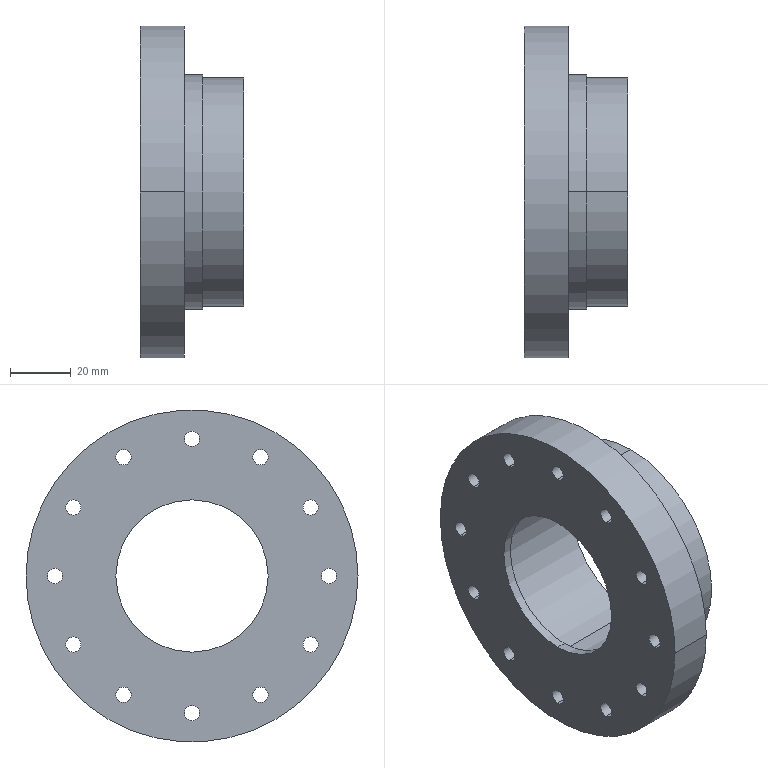Part | SolidWorks | features BaseBody 1, CirPattern 1, HoleWzd 1, ICE 1 | 1 solid | 55 faces | box 34 x 109 x 109 mm | volume 138553 mm3 | cylinder 42 | cone 8 | plane 5 | commonest cylinder face diameters 5 x32 50 x2 55 x2 75 x2 77 x2 109 x2